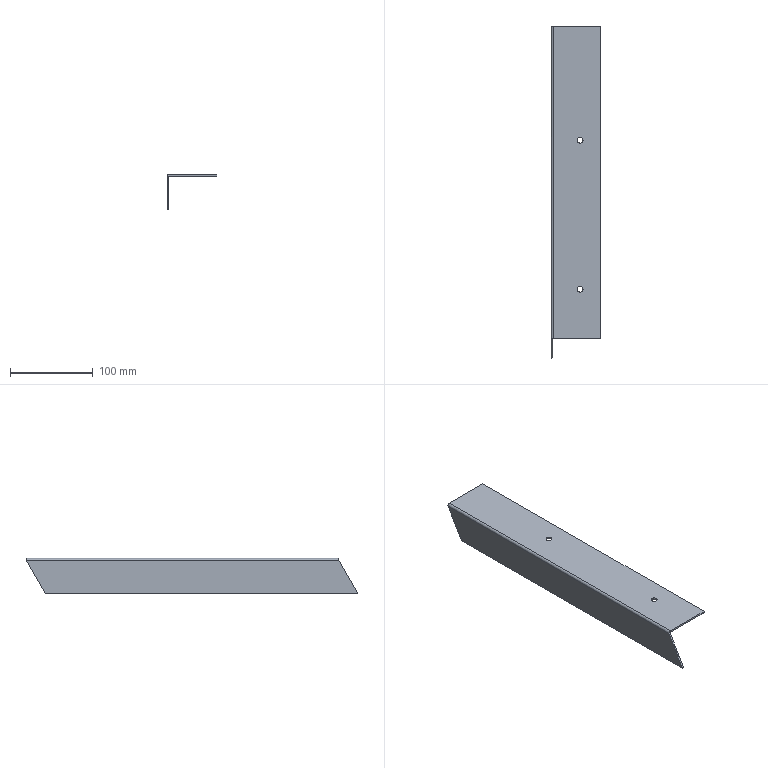Part | STEP file | zzf001-2 | 1 solid | 17 faces | box 60 x 401.094 x 42.5 mm | volume 75314 mm3 | plane 10 | cylinder 6 | spline 1 | commonest cylinder face diameters 7 x4 1 x1 5 x1
STEP:
#1=CARTESIAN_POINT('',(10.017,-69.969,0.));
#2=VERTEX_POINT('',#1);
#3=CARTESIAN_POINT('',(3.017,-69.969,0.));
#4=VERTEX_POINT('',#3);
#5=CARTESIAN_POINT('',(6.517,-69.969,0.));
#6=DIRECTION('',(0.,0.,-1.));
#7=DIRECTION('',(-1.,0.,0.));
#8=AXIS2_PLACEMENT_3D('',#5,#6,#7);
#9=CIRCLE('',#8,3.5);
#10=EDGE_CURVE('',#2,#4,#9,.T.);
#11=ORIENTED_EDGE('',*,*,#10,.F.);
#12=CARTESIAN_POINT('',(10.017,-69.969,-2.));
#13=VERTEX_POINT('',#12);
#14=CARTESIAN_POINT('',(10.017,-69.969,8.));
#15=DIRECTION('',(0.,0.,-1.));
#16=VECTOR('',#15,1000.);
#17=LINE('',#14,#16);
#18=EDGE_CURVE('',#2,#13,#17,.T.);
#19=ORIENTED_EDGE('',*,*,#18,.T.);
#20=CARTESIAN_POINT('',(3.017,-69.969,-2.));
#21=VERTEX_POINT('',#20);
#22=CARTESIAN_POINT('',(6.517,-69.969,-2.));
#23=DIRECTION('',(0.,0.,1.));
#24=DIRECTION('',(-1.,0.,0.));
#25=AXIS2_PLACEMENT_3D('',#22,#23,#24);
#26=CIRCLE('',#25,3.5);
#27=EDGE_CURVE('',#21,#13,#26,.T.);
#28=ORIENTED_EDGE('',*,*,#27,.F.);
#29=CARTESIAN_POINT('',(3.017,-69.969,8.));
#30=DIRECTION('',(0.,0.,-1.));
#31=VECTOR('',#30,1000.);
#32=LINE('',#29,#31);
#33=EDGE_CURVE('',#4,#21,#32,.T.);
#34=ORIENTED_EDGE('',*,*,#33,.F.);
#35=EDGE_LOOP('',(#11,#19,#28,#34));
#36=FACE_OUTER_BOUND('',#35,.T.);
#37=CARTESIAN_POINT('',(6.517,-69.969,8.));
#38=DIRECTION('',(0.,0.,-1.));
#39=DIRECTION('',(-1.,0.,0.));
#40=AXIS2_PLACEMENT_3D('',#37,#38,#39);
#41=CYLINDRICAL_SURFACE('',#40,3.5);
#42=ADVANCED_FACE('',(#36),#41,.F.);
#43=CARTESIAN_POINT('',(10.017,-249.969,0.));
#44=VERTEX_POINT('',#43);
#45=CARTESIAN_POINT('',(3.017,-249.969,0.));
#46=VERTEX_POINT('',#45);
#47=CARTESIAN_POINT('',(6.517,-249.969,0.));
#48=DIRECTION('',(0.,0.,-1.));
#49=DIRECTION('',(-1.,0.,0.));
#50=AXIS2_PLACEMENT_3D('',#47,#48,#49);
#51=CIRCLE('',#50,3.5);
#52=EDGE_CURVE('',#44,#46,#51,.T.);
#53=ORIENTED_EDGE('',*,*,#52,.F.);
#54=CARTESIAN_POINT('',(10.017,-249.969,-2.));
#55=VERTEX_POINT('',#54);
#56=CARTESIAN_POINT('',(10.017,-249.969,8.));
#57=DIRECTION('',(0.,0.,-1.));
#58=VECTOR('',#57,1000.);
#59=LINE('',#56,#58);
#60=EDGE_CURVE('',#44,#55,#59,.T.);
#61=ORIENTED_EDGE('',*,*,#60,.T.);
#62=CARTESIAN_POINT('',(3.017,-249.969,-2.));
#63=VERTEX_POINT('',#62);
#64=CARTESIAN_POINT('',(6.517,-249.969,-2.));
#65=DIRECTION('',(0.,0.,1.));
#66=DIRECTION('',(-1.,0.,0.));
#67=AXIS2_PLACEMENT_3D('',#64,#65,#66);
#68=CIRCLE('',#67,3.5);
#69=EDGE_CURVE('',#63,#55,#68,.T.);
#70=ORIENTED_EDGE('',*,*,#69,.F.);
#71=CARTESIAN_POINT('',(3.017,-249.969,8.));
#72=DIRECTION('',(0.,0.,-1.));
#73=VECTOR('',#72,1000.);
#74=LINE('',#71,#73);
#75=EDGE_CURVE('',#46,#63,#74,.T.);
#76=ORIENTED_EDGE('',*,*,#75,.F.);
#77=EDGE_LOOP('',(#53,#61,#70,#76));
#78=FACE_OUTER_BOUND('',#77,.T.);
#79=CARTESIAN_POINT('',(6.517,-249.969,8.));
#80=DIRECTION('',(0.,0.,-1.));
#81=DIRECTION('',(-1.,0.,0.));
#82=AXIS2_PLACEMENT_3D('',#79,#80,#81);
#83=CYLINDRICAL_SURFACE('',#82,3.5);
#84=ADVANCED_FACE('',(#78),#83,.F.);
#85=CARTESIAN_POINT('',(-25.983,-309.969,0.));
#86=VERTEX_POINT('',#85);
#87=CARTESIAN_POINT('',(31.517,-309.969,0.));
#88=VERTEX_POINT('',#87);
#89=CARTESIAN_POINT('',(0.,-309.969,0.));
#90=DIRECTION('',(1.,0.,0.));
#91=VECTOR('',#90,1000.);
#92=LINE('',#89,#91);
#93=EDGE_CURVE('',#86,#88,#92,.T.);
#94=ORIENTED_EDGE('',*,*,#93,.T.);
#95=CARTESIAN_POINT('',(31.517,68.031,0.));
#96=VERTEX_POINT('',#95);
#97=CARTESIAN_POINT('',(31.517,0.,0.));
#98=DIRECTION('',(0.,1.,0.));
#99=VECTOR('',#98,1000.);
#100=LINE('',#97,#99);
#101=EDGE_CURVE('',#88,#96,#100,.T.);
#102=ORIENTED_EDGE('',*,*,#101,.T.);
#103=CARTESIAN_POINT('',(-25.983,68.031,0.));
#104=VERTEX_POINT('',#103);
#105=CARTESIAN_POINT('',(0.,68.031,0.));
#106=DIRECTION('',(-1.,0.,0.));
#107=VECTOR('',#106,1000.);
#108=LINE('',#105,#107);
#109=EDGE_CURVE('',#96,#104,#108,.T.);
#110=ORIENTED_EDGE('',*,*,#109,.T.);
#111=CARTESIAN_POINT('',(-25.983,0.,0.));
#112=DIRECTION('',(0.,-1.,0.));
#113=VECTOR('',#112,1000.);
#114=LINE('',#111,#113);
#115=EDGE_CURVE('',#104,#86,#114,.T.);
#116=ORIENTED_EDGE('',*,*,#115,.T.);
#117=EDGE_LOOP('',(#94,#102,#110,#116));
#118=FACE_OUTER_BOUND('',#117,.T.);
#119=CARTESIAN_POINT('',(6.517,-69.969,0.));
#120=DIRECTION('',(0.,0.,-1.));
#121=DIRECTION('',(-1.,0.,0.));
#122=AXIS2_PLACEMENT_3D('',#119,#120,#121);
#123=CIRCLE('',#122,3.5);
#124=EDGE_CURVE('',#4,#2,#123,.T.);
#125=ORIENTED_EDGE('',*,*,#124,.T.);
#126=ORIENTED_EDGE('',*,*,#10,.T.);
#127=EDGE_LOOP('',(#125,#126));
#128=FACE_BOUND('',#127,.T.);
#129=CARTESIAN_POINT('',(6.517,-249.969,0.));
#130=DIRECTION('',(0.,0.,-1.));
#131=DIRECTION('',(-1.,0.,0.));
#132=AXIS2_PLACEMENT_3D('',#129,#130,#131);
#133=CIRCLE('',#132,3.5);
#134=EDGE_CURVE('',#46,#44,#133,.T.);
#135=ORIENTED_EDGE('',*,*,#134,.T.);
#136=ORIENTED_EDGE('',*,*,#52,.T.);
#137=EDGE_LOOP('',(#135,#136));
#138=FACE_BOUND('',#137,.T.);
#139=CARTESIAN_POINT('',(0.,0.,0.));
#140=DIRECTION('',(0.,0.,1.));
#141=DIRECTION('',(1.,0.,0.));
#142=AXIS2_PLACEMENT_3D('',#139,#140,#141);
#143=PLANE('',#142);
#144=ADVANCED_FACE('',(#118,#128,#138),#143,.T.);
#145=CARTESIAN_POINT('',(31.517,-309.969,-2.));
#146=VERTEX_POINT('',#145);
#147=CARTESIAN_POINT('',(31.517,68.031,-2.));
#148=VERTEX_POINT('',#147);
#149=CARTESIAN_POINT('',(31.517,68.031,-2.));
#150=DIRECTION('',(0.,1.,0.));
#151=VECTOR('',#150,1000.);
#152=LINE('',#149,#151);
#153=EDGE_CURVE('',#146,#148,#152,.T.);
#154=ORIENTED_EDGE('',*,*,#153,.T.);
#155=CARTESIAN_POINT('',(31.517,68.031,-2.));
#156=DIRECTION('',(0.,0.,1.));
#157=VECTOR('',#156,1000.);
#158=LINE('',#155,#157);
#159=EDGE_CURVE('',#148,#96,#158,.T.);
#160=ORIENTED_EDGE('',*,*,#159,.T.);
#161=ORIENTED_EDGE('',*,*,#101,.F.);
#162=CARTESIAN_POINT('',(31.517,-309.969,-2.));
#163=DIRECTION('',(0.,0.,-1.));
#164=VECTOR('',#163,1000.);
#165=LINE('',#162,#164);
#166=EDGE_CURVE('',#88,#146,#165,.T.);
#167=ORIENTED_EDGE('',*,*,#166,.T.);
#168=EDGE_LOOP('',(#154,#160,#161,#167));
#169=FACE_OUTER_BOUND('',#168,.T.);
#170=CARTESIAN_POINT('',(31.517,68.031,-2.));
#171=DIRECTION('',(1.,0.,0.));
#172=DIRECTION('',(0.,1.,0.));
#173=AXIS2_PLACEMENT_3D('',#170,#171,#172);
#174=PLANE('',#173);
#175=ADVANCED_FACE('',(#169),#174,.T.);
#176=ORIENTED_EDGE('',*,*,#166,.F.);
#177=ORIENTED_EDGE('',*,*,#93,.F.);
#178=CARTESIAN_POINT('',(-28.483,-309.969,-2.5));
#179=VERTEX_POINT('',#178);
#180=CARTESIAN_POINT('',(-25.983,-309.969,-2.5));
#181=DIRECTION('',(0.,1.,0.));
#182=DIRECTION('',(0.,0.,1.));
#183=AXIS2_PLACEMENT_3D('',#180,#181,#182);
#184=CIRCLE('',#183,2.5);
#185=EDGE_CURVE('',#179,#86,#184,.T.);
#186=ORIENTED_EDGE('',*,*,#185,.F.);
#187=CARTESIAN_POINT('',(-26.483,-309.969,-2.5));
#188=VERTEX_POINT('',#187);
#189=CARTESIAN_POINT('',(-25.983,-309.969,-2.5));
#190=DIRECTION('',(1.,0.,0.));
#191=VECTOR('',#190,1000.);
#192=LINE('',#189,#191);
#193=EDGE_CURVE('',#179,#188,#192,.T.);
#194=ORIENTED_EDGE('',*,*,#193,.T.);
#195=CARTESIAN_POINT('',(-25.983,-309.969,-2.));
#196=VERTEX_POINT('',#195);
#197=CARTESIAN_POINT('',(-25.983,-309.969,-2.5));
#198=DIRECTION('',(0.,1.,0.));
#199=DIRECTION('',(0.,0.,1.));
#200=AXIS2_PLACEMENT_3D('',#197,#198,#199);
#201=CIRCLE('',#200,0.5);
#202=EDGE_CURVE('',#188,#196,#201,.T.);
#203=ORIENTED_EDGE('',*,*,#202,.T.);
#204=CARTESIAN_POINT('',(-26.483,-309.969,-2.));
#205=DIRECTION('',(1.,0.,0.));
#206=VECTOR('',#205,1000.);
#207=LINE('',#204,#206);
#208=EDGE_CURVE('',#196,#146,#207,.T.);
#209=ORIENTED_EDGE('',*,*,#208,.T.);
#210=EDGE_LOOP('',(#176,#177,#186,#194,#203,#209));
#211=FACE_OUTER_BOUND('',#210,.T.);
#212=CARTESIAN_POINT('',(-26.483,-309.969,-2.));
#213=DIRECTION('',(0.,-1.,0.));
#214=DIRECTION('',(0.,0.,-1.));
#215=AXIS2_PLACEMENT_3D('',#212,#213,#214);
#216=PLANE('',#215);
#217=ADVANCED_FACE('',(#211),#216,.T.);
#218=CARTESIAN_POINT('',(-28.483,67.743,-2.5));
#219=VERTEX_POINT('',#218);
#220=CARTESIAN_POINT('',(-28.483,68.031,-2.5));
#221=DIRECTION('',(0.,-1.,0.));
#222=VECTOR('',#221,1000.);
#223=LINE('',#220,#222);
#224=EDGE_CURVE('',#219,#179,#223,.T.);
#225=ORIENTED_EDGE('',*,*,#224,.T.);
#226=ORIENTED_EDGE('',*,*,#185,.T.);
#227=ORIENTED_EDGE('',*,*,#115,.F.);
#228=CARTESIAN_POINT('',(-25.983,68.031,0.));
#229=CARTESIAN_POINT('',(-26.31,68.007,0.));
#230=CARTESIAN_POINT('',(-26.637,67.983,-0.06507));
#231=CARTESIAN_POINT('',(-27.242,67.935,-0.3155));
#232=CARTESIAN_POINT('',(-27.519,67.911,-0.5008));
#233=CARTESIAN_POINT('',(-27.982,67.863,-0.9636));
#234=CARTESIAN_POINT('',(-28.167,67.839,-1.241));
#235=CARTESIAN_POINT('',(-28.418,67.791,-1.846));
#236=CARTESIAN_POINT('',(-28.483,67.767,-2.173));
#237=CARTESIAN_POINT('',(-28.483,67.743,-2.5));
#238=B_SPLINE_CURVE_WITH_KNOTS('',3,(#228,#229,#230,#231,#232,#233,#234,#235,#236,#237),.UNSPECIFIED.,.F.,.F.,(4,2,2,2,4),(0.,0.25,0.5,0.75,1.),.UNSPECIFIED.);
#239=EDGE_CURVE('',#104,#219,#238,.T.);
#240=ORIENTED_EDGE('',*,*,#239,.T.);
#241=EDGE_LOOP('',(#225,#226,#227,#240));
#242=FACE_OUTER_BOUND('',#241,.T.);
#243=CARTESIAN_POINT('',(-25.983,68.031,-2.5));
#244=DIRECTION('',(0.,1.,0.));
#245=DIRECTION('',(0.,0.,1.));
#246=AXIS2_PLACEMENT_3D('',#243,#244,#245);
#247=CYLINDRICAL_SURFACE('',#246,2.5);
#248=ADVANCED_FACE('',(#242),#247,.T.);
#249=ORIENTED_EDGE('',*,*,#109,.F.);
#250=ORIENTED_EDGE('',*,*,#159,.F.);
#251=CARTESIAN_POINT('',(-25.983,68.031,-2.));
#252=VERTEX_POINT('',#251);
#253=CARTESIAN_POINT('',(-26.483,68.031,-2.));
#254=DIRECTION('',(-1.,0.,0.));
#255=VECTOR('',#254,1000.);
#256=LINE('',#253,#255);
#257=EDGE_CURVE('',#148,#252,#256,.T.);
#258=ORIENTED_EDGE('',*,*,#257,.T.);
#259=CARTESIAN_POINT('',(-25.983,68.031,-2.));
#260=DIRECTION('',(0.,0.,1.));
#261=VECTOR('',#260,1000.);
#262=LINE('',#259,#261);
#263=EDGE_CURVE('',#252,#104,#262,.T.);
#264=ORIENTED_EDGE('',*,*,#263,.T.);
#265=EDGE_LOOP('',(#249,#250,#258,#264));
#266=FACE_OUTER_BOUND('',#265,.T.);
#267=CARTESIAN_POINT('',(-26.483,68.031,-2.));
#268=DIRECTION('',(0.,1.,0.));
#269=DIRECTION('',(0.,0.,1.));
#270=AXIS2_PLACEMENT_3D('',#267,#268,#269);
#271=PLANE('',#270);
#272=ADVANCED_FACE('',(#266),#271,.T.);
#273=ORIENTED_EDGE('',*,*,#18,.F.);
#274=ORIENTED_EDGE('',*,*,#124,.F.);
#275=ORIENTED_EDGE('',*,*,#33,.T.);
#276=CARTESIAN_POINT('',(6.517,-69.969,-2.));
#277=DIRECTION('',(0.,0.,1.));
#278=DIRECTION('',(-1.,0.,0.));
#279=AXIS2_PLACEMENT_3D('',#276,#277,#278);
#280=CIRCLE('',#279,3.5);
#281=EDGE_CURVE('',#13,#21,#280,.T.);
#282=ORIENTED_EDGE('',*,*,#281,.F.);
#283=EDGE_LOOP('',(#273,#274,#275,#282));
#284=FACE_OUTER_BOUND('',#283,.T.);
#285=CARTESIAN_POINT('',(6.517,-69.969,8.));
#286=DIRECTION('',(0.,0.,-1.));
#287=DIRECTION('',(-1.,0.,0.));
#288=AXIS2_PLACEMENT_3D('',#285,#286,#287);
#289=CYLINDRICAL_SURFACE('',#288,3.5);
#290=ADVANCED_FACE('',(#284),#289,.F.);
#291=ORIENTED_EDGE('',*,*,#60,.F.);
#292=ORIENTED_EDGE('',*,*,#134,.F.);
#293=ORIENTED_EDGE('',*,*,#75,.T.);
#294=CARTESIAN_POINT('',(6.517,-249.969,-2.));
#295=DIRECTION('',(0.,0.,1.));
#296=DIRECTION('',(-1.,0.,0.));
#297=AXIS2_PLACEMENT_3D('',#294,#295,#296);
#298=CIRCLE('',#297,3.5);
#299=EDGE_CURVE('',#55,#63,#298,.T.);
#300=ORIENTED_EDGE('',*,*,#299,.F.);
#301=EDGE_LOOP('',(#291,#292,#293,#300));
#302=FACE_OUTER_BOUND('',#301,.T.);
#303=CARTESIAN_POINT('',(6.517,-249.969,8.));
#304=DIRECTION('',(0.,0.,-1.));
#305=DIRECTION('',(-1.,0.,0.));
#306=AXIS2_PLACEMENT_3D('',#303,#304,#305);
#307=CYLINDRICAL_SURFACE('',#306,3.5);
#308=ADVANCED_FACE('',(#302),#307,.F.);
#309=ORIENTED_EDGE('',*,*,#257,.F.);
#310=ORIENTED_EDGE('',*,*,#153,.F.);
#311=ORIENTED_EDGE('',*,*,#208,.F.);
#312=CARTESIAN_POINT('',(-25.983,0.,-2.));
#313=DIRECTION('',(0.,-1.,0.));
#314=VECTOR('',#313,1000.);
#315=LINE('',#312,#314);
#316=EDGE_CURVE('',#252,#196,#315,.T.);
#317=ORIENTED_EDGE('',*,*,#316,.F.);
#318=EDGE_LOOP('',(#309,#310,#311,#317));
#319=FACE_OUTER_BOUND('',#318,.T.);
#320=ORIENTED_EDGE('',*,*,#27,.T.);
#321=ORIENTED_EDGE('',*,*,#281,.T.);
#322=EDGE_LOOP('',(#320,#321));
#323=FACE_BOUND('',#322,.T.);
#324=ORIENTED_EDGE('',*,*,#69,.T.);
#325=ORIENTED_EDGE('',*,*,#299,.T.);
#326=EDGE_LOOP('',(#324,#325));
#327=FACE_BOUND('',#326,.T.);
#328=CARTESIAN_POINT('',(0.,0.,-2.));
#329=DIRECTION('',(0.,0.,1.));
#330=DIRECTION('',(1.,0.,0.));
#331=AXIS2_PLACEMENT_3D('',#328,#329,#330);
#332=PLANE('',#331);
#333=ADVANCED_FACE('',(#319,#323,#327),#332,.F.);
#334=ORIENTED_EDGE('',*,*,#224,.F.);
#335=CARTESIAN_POINT('',(-28.483,44.649,-42.5));
#336=VERTEX_POINT('',#335);
#337=CARTESIAN_POINT('',(-28.483,67.743,-2.5));
#338=DIRECTION('',(0.,-0.5,-0.866));
#339=VECTOR('',#338,1000.);
#340=LINE('',#337,#339);
#341=EDGE_CURVE('',#219,#336,#340,.T.);
#342=ORIENTED_EDGE('',*,*,#341,.T.);
#343=CARTESIAN_POINT('',(-28.483,-333.063,-42.5));
#344=VERTEX_POINT('',#343);
#345=CARTESIAN_POINT('',(-28.483,0.,-42.5));
#346=DIRECTION('',(0.,-1.,0.));
#347=VECTOR('',#346,1000.);
#348=LINE('',#345,#347);
#349=EDGE_CURVE('',#336,#344,#348,.T.);
#350=ORIENTED_EDGE('',*,*,#349,.T.);
#351=CARTESIAN_POINT('',(-28.483,-333.063,-42.5));
#352=DIRECTION('',(0.,0.5,0.866));
#353=VECTOR('',#352,1000.);
#354=LINE('',#351,#353);
#355=EDGE_CURVE('',#344,#179,#354,.T.);
#356=ORIENTED_EDGE('',*,*,#355,.T.);
#357=EDGE_LOOP('',(#334,#342,#350,#356));
#358=FACE_OUTER_BOUND('',#357,.T.);
#359=CARTESIAN_POINT('',(-28.483,0.,0.));
#360=DIRECTION('',(-1.,0.,0.));
#361=DIRECTION('',(0.,0.,1.));
#362=AXIS2_PLACEMENT_3D('',#359,#360,#361);
#363=PLANE('',#362);
#364=ADVANCED_FACE('',(#358),#363,.T.);
#365=CARTESIAN_POINT('',(-26.483,67.743,-2.5));
#366=VERTEX_POINT('',#365);
#367=CARTESIAN_POINT('',(-27.483,67.743,-2.5));
#368=DIRECTION('',(1.,0.,0.));
#369=VECTOR('',#368,1000.);
#370=LINE('',#367,#369);
#371=EDGE_CURVE('',#219,#366,#370,.T.);
#372=ORIENTED_EDGE('',*,*,#371,.F.);
#373=ORIENTED_EDGE('',*,*,#239,.F.);
#374=ORIENTED_EDGE('',*,*,#263,.F.);
#375=CARTESIAN_POINT('',(-26.483,67.743,-2.5));
#376=CARTESIAN_POINT('',(-26.483,67.791,-2.369));
#377=CARTESIAN_POINT('',(-26.429,67.839,-2.239));
#378=CARTESIAN_POINT('',(-26.244,67.935,-2.054));
#379=CARTESIAN_POINT('',(-26.114,67.983,-2.));
#380=CARTESIAN_POINT('',(-25.983,68.031,-2.));
#381=B_SPLINE_CURVE_WITH_KNOTS('',3,(#375,#376,#377,#378,#379,#380),.UNSPECIFIED.,.F.,.F.,(4,2,4),(0.,0.5,1.),.UNSPECIFIED.);
#382=EDGE_CURVE('',#366,#252,#381,.T.);
#383=ORIENTED_EDGE('',*,*,#382,.F.);
#384=EDGE_LOOP('',(#372,#373,#374,#383));
#385=FACE_OUTER_BOUND('',#384,.T.);
#386=CARTESIAN_POINT('',(-28.503,67.743,-2.5));
#387=CARTESIAN_POINT('',(-28.503,67.767,-2.17));
#388=CARTESIAN_POINT('',(-28.437,67.791,-1.84));
#389=CARTESIAN_POINT('',(-28.185,67.839,-1.231));
#390=CARTESIAN_POINT('',(-27.998,67.863,-0.9513));
#391=CARTESIAN_POINT('',(-27.531,67.911,-0.4848));
#392=CARTESIAN_POINT('',(-27.252,67.935,-0.2981));
#393=CARTESIAN_POINT('',(-26.642,67.983,-0.04559));
#394=CARTESIAN_POINT('',(-26.313,68.007,0.02));
#395=CARTESIAN_POINT('',(-25.983,68.031,0.02));
#396=CARTESIAN_POINT('',(-28.483,67.743,-2.5));
#397=CARTESIAN_POINT('',(-28.483,67.767,-2.173));
#398=CARTESIAN_POINT('',(-28.418,67.791,-1.846));
#399=CARTESIAN_POINT('',(-28.167,67.839,-1.241));
#400=CARTESIAN_POINT('',(-27.982,67.863,-0.9636));
#401=CARTESIAN_POINT('',(-27.519,67.911,-0.5008));
#402=CARTESIAN_POINT('',(-27.242,67.935,-0.3155));
#403=CARTESIAN_POINT('',(-26.637,67.983,-0.06507));
#404=CARTESIAN_POINT('',(-26.31,68.007,0.));
#405=CARTESIAN_POINT('',(-25.983,68.031,0.));
#406=CARTESIAN_POINT('',(-26.483,67.743,-2.5));
#407=CARTESIAN_POINT('',(-26.483,67.767,-2.435));
#408=CARTESIAN_POINT('',(-26.47,67.791,-2.369));
#409=CARTESIAN_POINT('',(-26.42,67.839,-2.248));
#410=CARTESIAN_POINT('',(-26.383,67.863,-2.193));
#411=CARTESIAN_POINT('',(-26.29,67.911,-2.1));
#412=CARTESIAN_POINT('',(-26.234,67.935,-2.063));
#413=CARTESIAN_POINT('',(-26.114,67.983,-2.013));
#414=CARTESIAN_POINT('',(-26.048,68.007,-2.));
#415=CARTESIAN_POINT('',(-25.983,68.031,-2.));
#416=CARTESIAN_POINT('',(-26.462,67.743,-2.5));
#417=CARTESIAN_POINT('',(-26.462,67.767,-2.437));
#418=CARTESIAN_POINT('',(-26.45,67.791,-2.374));
#419=CARTESIAN_POINT('',(-26.402,67.839,-2.258));
#420=CARTESIAN_POINT('',(-26.366,67.863,-2.205));
#421=CARTESIAN_POINT('',(-26.278,67.911,-2.116));
#422=CARTESIAN_POINT('',(-26.224,67.935,-2.081));
#423=CARTESIAN_POINT('',(-26.108,67.983,-2.033));
#424=CARTESIAN_POINT('',(-26.045,68.007,-2.02));
#425=CARTESIAN_POINT('',(-25.983,68.031,-2.02));
#426=B_SPLINE_SURFACE_WITH_KNOTS('',1,3,((#386,#387,#388,#389,#390,#391,#392,#393,#394,#395),(#396,#397,#398,#399,#400,#401,#402,#403,#404,#405),(#406,#407,#408,#409,#410,#411,#412,#413,#414,#415),(#416,#417,#418,#419,#420,#421,#422,#423,#424,#425)),.UNSPECIFIED.,.F.,.F.,.F.,(2,1,1,2),(4,2,2,2,4),(-0.01,0.,1.,1.01),(0.,0.25,0.5,0.75,1.),.UNSPECIFIED.);
#427=ADVANCED_FACE('',(#385),#426,.F.);
#428=ORIENTED_EDGE('',*,*,#202,.F.);
#429=CARTESIAN_POINT('',(-26.483,68.031,-2.5));
#430=DIRECTION('',(0.,-1.,0.));
#431=VECTOR('',#430,1000.);
#432=LINE('',#429,#431);
#433=EDGE_CURVE('',#366,#188,#432,.T.);
#434=ORIENTED_EDGE('',*,*,#433,.F.);
#435=ORIENTED_EDGE('',*,*,#382,.T.);
#436=ORIENTED_EDGE('',*,*,#316,.T.);
#437=EDGE_LOOP('',(#428,#434,#435,#436));
#438=FACE_OUTER_BOUND('',#437,.T.);
#439=CARTESIAN_POINT('',(-25.983,68.031,-2.5));
#440=DIRECTION('',(0.,1.,0.));
#441=DIRECTION('',(0.,0.,1.));
#442=AXIS2_PLACEMENT_3D('',#439,#440,#441);
#443=CYLINDRICAL_SURFACE('',#442,0.5);
#444=ADVANCED_FACE('',(#438),#443,.F.);
#445=ORIENTED_EDGE('',*,*,#355,.F.);
#446=CARTESIAN_POINT('',(-26.483,-333.063,-42.5));
#447=VERTEX_POINT('',#446);
#448=CARTESIAN_POINT('',(-28.483,-333.063,-42.5));
#449=DIRECTION('',(1.,0.,0.));
#450=VECTOR('',#449,1000.);
#451=LINE('',#448,#450);
#452=EDGE_CURVE('',#344,#447,#451,.T.);
#453=ORIENTED_EDGE('',*,*,#452,.T.);
#454=CARTESIAN_POINT('',(-26.483,-333.063,-42.5));
#455=DIRECTION('',(0.,0.5,0.866));
#456=VECTOR('',#455,1000.);
#457=LINE('',#454,#456);
#458=EDGE_CURVE('',#447,#188,#457,.T.);
#459=ORIENTED_EDGE('',*,*,#458,.T.);
#460=ORIENTED_EDGE('',*,*,#193,.F.);
#461=EDGE_LOOP('',(#445,#453,#459,#460));
#462=FACE_OUTER_BOUND('',#461,.T.);
#463=CARTESIAN_POINT('',(-28.483,-333.063,-42.5));
#464=DIRECTION('',(0.,-0.866,0.5));
#465=DIRECTION('',(0.,-0.5,-0.866));
#466=AXIS2_PLACEMENT_3D('',#463,#464,#465);
#467=PLANE('',#466);
#468=ADVANCED_FACE('',(#462),#467,.T.);
#469=CARTESIAN_POINT('',(-26.483,44.649,-42.5));
#470=VERTEX_POINT('',#469);
#471=CARTESIAN_POINT('',(-26.483,68.031,-2.));
#472=DIRECTION('',(0.,-0.5,-0.866));
#473=VECTOR('',#472,1000.);
#474=LINE('',#471,#473);
#475=EDGE_CURVE('',#366,#470,#474,.T.);
#476=ORIENTED_EDGE('',*,*,#475,.T.);
#477=CARTESIAN_POINT('',(-28.483,44.649,-42.5));
#478=DIRECTION('',(-1.,0.,0.));
#479=VECTOR('',#478,1000.);
#480=LINE('',#477,#479);
#481=EDGE_CURVE('',#470,#336,#480,.T.);
#482=ORIENTED_EDGE('',*,*,#481,.T.);
#483=ORIENTED_EDGE('',*,*,#341,.F.);
#484=ORIENTED_EDGE('',*,*,#371,.T.);
#485=EDGE_LOOP('',(#476,#482,#483,#484));
#486=FACE_OUTER_BOUND('',#485,.T.);
#487=CARTESIAN_POINT('',(-28.483,68.031,-2.));
#488=DIRECTION('',(0.,0.866,-0.5));
#489=DIRECTION('',(0.,0.5,0.866));
#490=AXIS2_PLACEMENT_3D('',#487,#488,#489);
#491=PLANE('',#490);
#492=ADVANCED_FACE('',(#486),#491,.T.);
#493=ORIENTED_EDGE('',*,*,#349,.F.);
#494=ORIENTED_EDGE('',*,*,#481,.F.);
#495=CARTESIAN_POINT('',(-26.483,44.649,-42.5));
#496=DIRECTION('',(0.,-1.,0.));
#497=VECTOR('',#496,1000.);
#498=LINE('',#495,#497);
#499=EDGE_CURVE('',#470,#447,#498,.T.);
#500=ORIENTED_EDGE('',*,*,#499,.T.);
#501=ORIENTED_EDGE('',*,*,#452,.F.);
#502=EDGE_LOOP('',(#493,#494,#500,#501));
#503=FACE_OUTER_BOUND('',#502,.T.);
#504=CARTESIAN_POINT('',(-28.483,44.649,-42.5));
#505=DIRECTION('',(0.,0.,-1.));
#506=DIRECTION('',(-1.,0.,0.));
#507=AXIS2_PLACEMENT_3D('',#504,#505,#506);
#508=PLANE('',#507);
#509=ADVANCED_FACE('',(#503),#508,.T.);
#510=ORIENTED_EDGE('',*,*,#458,.F.);
#511=ORIENTED_EDGE('',*,*,#499,.F.);
#512=ORIENTED_EDGE('',*,*,#475,.F.);
#513=ORIENTED_EDGE('',*,*,#433,.T.);
#514=EDGE_LOOP('',(#510,#511,#512,#513));
#515=FACE_OUTER_BOUND('',#514,.T.);
#516=CARTESIAN_POINT('',(-26.483,0.,0.));
#517=DIRECTION('',(-1.,0.,0.));
#518=DIRECTION('',(0.,0.,1.));
#519=AXIS2_PLACEMENT_3D('',#516,#517,#518);
#520=PLANE('',#519);
#521=ADVANCED_FACE('',(#515),#520,.F.);
#522=CLOSED_SHELL('',(#42,#84,#144,#175,#217,#248,#272,#290,#308,#333,#364,#427,#444,#468,#492,#509,#521));
#523=MANIFOLD_SOLID_BREP('',#522);
#524=CARTESIAN_POINT('',(0.,0.,0.));
#525=DIRECTION('',(0.,0.,1.));
#526=DIRECTION('',(1.,0.,0.));
#527=AXIS2_PLACEMENT_3D('',#524,#525,#526);
#528=(LENGTH_UNIT()NAMED_UNIT(*)SI_UNIT(.MILLI.,.METRE.));
#529=UNCERTAINTY_MEASURE_WITH_UNIT(LENGTH_MEASURE(0.00001),#528,'','');
#530=(NAMED_UNIT(*)PLANE_ANGLE_UNIT()SI_UNIT($,.RADIAN.));
#531=(NAMED_UNIT(*)SI_UNIT($,.STERADIAN.)SOLID_ANGLE_UNIT());
#532=(GEOMETRIC_REPRESENTATION_CONTEXT(3)GLOBAL_UNCERTAINTY_ASSIGNED_CONTEXT((#529))GLOBAL_UNIT_ASSIGNED_CONTEXT((#528,#530,#531))REPRESENTATION_CONTEXT('',''));
#533=ADVANCED_BREP_SHAPE_REPRESENTATION('',(#523,#527),#532);